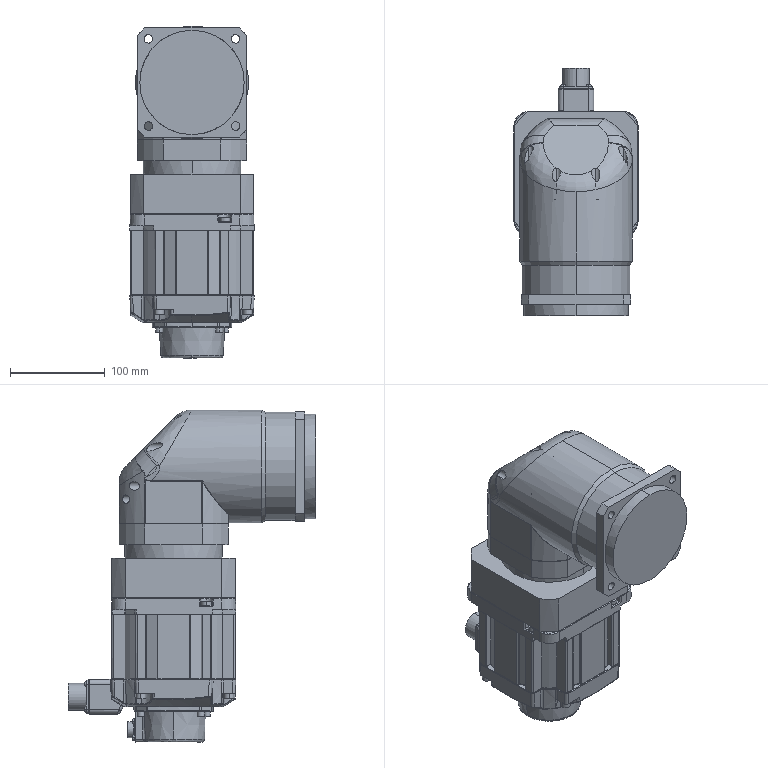Part | SolidWorks | features BaseBody 2, CombineBodies 1 | 1 solid | 1160 faces | box 130.933 x 261.25 x 349.9 mm | volume 4855560 mm3 | cylinder 428 | plane 341 | spline 215 | cone 148 | torus 28 | commonest cylinder face diameters 1 x81 3 x42 6 x37 2 x31 9 x28 128.5 x24